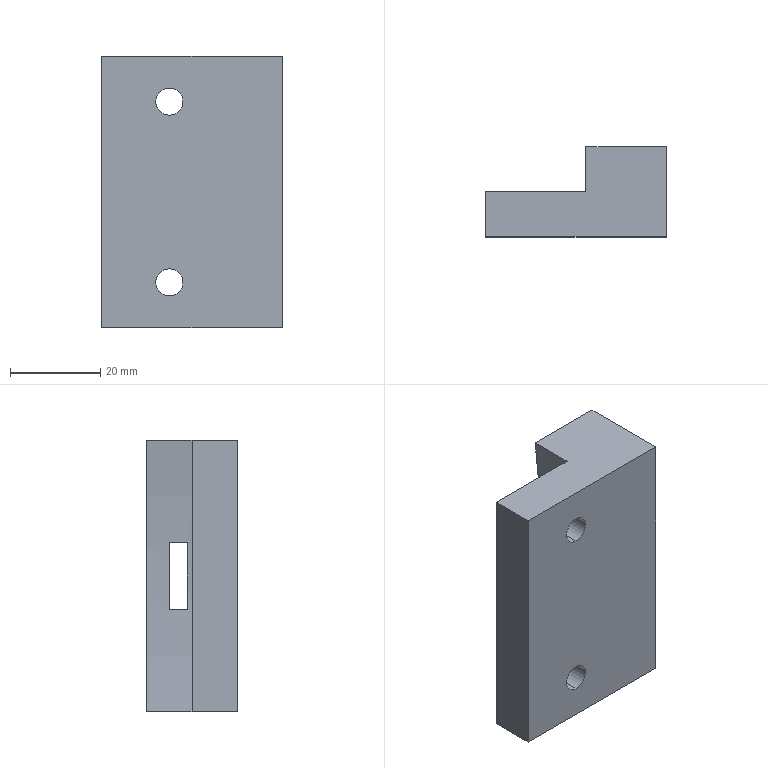Part | SolidWorks | features ICE 3, Extrusion 1 | 1 solid | 16 faces | box 40 x 20 x 60 mm | volume 32417 mm3 | plane 11 | cylinder 5 | commonest cylinder face diameters 6 x4 490 x1
STEP:
#1=CARTESIAN_POINT('',(15.,-20.,7.));
#2=VERTEX_POINT('',#1);
#3=CARTESIAN_POINT('',(15.,-20.,13.));
#4=VERTEX_POINT('',#3);
#5=CARTESIAN_POINT('',(15.,-20.,10.));
#6=DIRECTION('',(0.,1.,0.));
#7=DIRECTION('',(0.,0.,1.));
#8=AXIS2_PLACEMENT_3D('',#5,#6,#7);
#9=CIRCLE('',#8,3.);
#10=EDGE_CURVE('',#2,#4,#9,.T.);
#11=ORIENTED_EDGE('',*,*,#10,.F.);
#12=CARTESIAN_POINT('',(15.,-10.,7.));
#13=VERTEX_POINT('',#12);
#14=CARTESIAN_POINT('',(15.,-20.,7.));
#15=DIRECTION('',(0.,1.,0.));
#16=VECTOR('',#15,1000.);
#17=LINE('',#14,#16);
#18=EDGE_CURVE('',#2,#13,#17,.T.);
#19=ORIENTED_EDGE('',*,*,#18,.T.);
#20=CARTESIAN_POINT('',(15.,-10.,13.));
#21=VERTEX_POINT('',#20);
#22=CARTESIAN_POINT('',(15.,-10.,10.));
#23=DIRECTION('',(0.,1.,0.));
#24=DIRECTION('',(0.,0.,1.));
#25=AXIS2_PLACEMENT_3D('',#22,#23,#24);
#26=CIRCLE('',#25,3.);
#27=EDGE_CURVE('',#13,#21,#26,.T.);
#28=ORIENTED_EDGE('',*,*,#27,.T.);
#29=CARTESIAN_POINT('',(15.,-20.,13.));
#30=DIRECTION('',(0.,1.,0.));
#31=VECTOR('',#30,1000.);
#32=LINE('',#29,#31);
#33=EDGE_CURVE('',#4,#21,#32,.T.);
#34=ORIENTED_EDGE('',*,*,#33,.F.);
#35=EDGE_LOOP('',(#11,#19,#28,#34));
#36=FACE_OUTER_BOUND('',#35,.T.);
#37=CARTESIAN_POINT('',(15.,-20.,10.));
#38=DIRECTION('',(0.,1.,0.));
#39=DIRECTION('',(0.,0.,1.));
#40=AXIS2_PLACEMENT_3D('',#37,#38,#39);
#41=CYLINDRICAL_SURFACE('',#40,3.);
#42=ADVANCED_FACE('',(#36),#41,.F.);
#43=CARTESIAN_POINT('',(15.,-20.,47.));
#44=VERTEX_POINT('',#43);
#45=CARTESIAN_POINT('',(15.,-20.,53.));
#46=VERTEX_POINT('',#45);
#47=CARTESIAN_POINT('',(15.,-20.,50.));
#48=DIRECTION('',(0.,1.,0.));
#49=DIRECTION('',(0.,0.,1.));
#50=AXIS2_PLACEMENT_3D('',#47,#48,#49);
#51=CIRCLE('',#50,3.);
#52=EDGE_CURVE('',#44,#46,#51,.T.);
#53=ORIENTED_EDGE('',*,*,#52,.F.);
#54=CARTESIAN_POINT('',(15.,-10.,47.));
#55=VERTEX_POINT('',#54);
#56=CARTESIAN_POINT('',(15.,-20.,47.));
#57=DIRECTION('',(0.,1.,0.));
#58=VECTOR('',#57,1000.);
#59=LINE('',#56,#58);
#60=EDGE_CURVE('',#44,#55,#59,.T.);
#61=ORIENTED_EDGE('',*,*,#60,.T.);
#62=CARTESIAN_POINT('',(15.,-10.,53.));
#63=VERTEX_POINT('',#62);
#64=CARTESIAN_POINT('',(15.,-10.,50.));
#65=DIRECTION('',(0.,1.,0.));
#66=DIRECTION('',(0.,0.,1.));
#67=AXIS2_PLACEMENT_3D('',#64,#65,#66);
#68=CIRCLE('',#67,3.);
#69=EDGE_CURVE('',#55,#63,#68,.T.);
#70=ORIENTED_EDGE('',*,*,#69,.T.);
#71=CARTESIAN_POINT('',(15.,-20.,53.));
#72=DIRECTION('',(0.,1.,0.));
#73=VECTOR('',#72,1000.);
#74=LINE('',#71,#73);
#75=EDGE_CURVE('',#46,#63,#74,.T.);
#76=ORIENTED_EDGE('',*,*,#75,.F.);
#77=EDGE_LOOP('',(#53,#61,#70,#76));
#78=FACE_OUTER_BOUND('',#77,.T.);
#79=CARTESIAN_POINT('',(15.,-20.,50.));
#80=DIRECTION('',(0.,1.,0.));
#81=DIRECTION('',(0.,0.,1.));
#82=AXIS2_PLACEMENT_3D('',#79,#80,#81);
#83=CYLINDRICAL_SURFACE('',#82,3.);
#84=ADVANCED_FACE('',(#78),#83,.F.);
#85=CARTESIAN_POINT('',(40.,0.,0.));
#86=VERTEX_POINT('',#85);
#87=CARTESIAN_POINT('',(22.2,0.,0.));
#88=VERTEX_POINT('',#87);
#89=CARTESIAN_POINT('',(40.,0.,0.));
#90=DIRECTION('',(-1.,0.,0.));
#91=VECTOR('',#90,1000.);
#92=LINE('',#89,#91);
#93=EDGE_CURVE('',#86,#88,#92,.T.);
#94=ORIENTED_EDGE('',*,*,#93,.T.);
#95=CARTESIAN_POINT('',(22.2,0.,60.));
#96=VERTEX_POINT('',#95);
#97=CARTESIAN_POINT('',(-220.956,0.,30.));
#98=DIRECTION('',(0.,1.,0.));
#99=DIRECTION('',(0.,0.,-1.));
#100=AXIS2_PLACEMENT_3D('',#97,#98,#99);
#101=CIRCLE('',#100,245.);
#102=EDGE_CURVE('',#96,#88,#101,.T.);
#103=ORIENTED_EDGE('',*,*,#102,.F.);
#104=CARTESIAN_POINT('',(40.,0.,60.));
#105=VERTEX_POINT('',#104);
#106=CARTESIAN_POINT('',(40.,0.,60.));
#107=DIRECTION('',(-1.,0.,0.));
#108=VECTOR('',#107,1000.);
#109=LINE('',#106,#108);
#110=EDGE_CURVE('',#105,#96,#109,.T.);
#111=ORIENTED_EDGE('',*,*,#110,.F.);
#112=CARTESIAN_POINT('',(40.,0.,60.));
#113=DIRECTION('',(0.,0.,-1.));
#114=VECTOR('',#113,1000.);
#115=LINE('',#112,#114);
#116=EDGE_CURVE('',#105,#86,#115,.T.);
#117=ORIENTED_EDGE('',*,*,#116,.T.);
#118=EDGE_LOOP('',(#94,#103,#111,#117));
#119=FACE_OUTER_BOUND('',#118,.T.);
#120=CARTESIAN_POINT('',(40.,0.,60.));
#121=DIRECTION('',(0.,-1.,0.));
#122=DIRECTION('',(0.,0.,-1.));
#123=AXIS2_PLACEMENT_3D('',#120,#121,#122);
#124=PLANE('',#123);
#125=ADVANCED_FACE('',(#119),#124,.F.);
#126=CARTESIAN_POINT('',(0.,-10.,60.));
#127=VERTEX_POINT('',#126);
#128=CARTESIAN_POINT('',(0.,-20.,60.));
#129=VERTEX_POINT('',#128);
#130=CARTESIAN_POINT('',(0.,0.,60.));
#131=DIRECTION('',(0.,-1.,0.));
#132=VECTOR('',#131,1000.);
#133=LINE('',#130,#132);
#134=EDGE_CURVE('',#127,#129,#133,.T.);
#135=ORIENTED_EDGE('',*,*,#134,.F.);
#136=CARTESIAN_POINT('',(0.,-10.,0.));
#137=VERTEX_POINT('',#136);
#138=CARTESIAN_POINT('',(0.,-10.,0.));
#139=DIRECTION('',(0.,0.,1.));
#140=VECTOR('',#139,1000.);
#141=LINE('',#138,#140);
#142=EDGE_CURVE('',#137,#127,#141,.T.);
#143=ORIENTED_EDGE('',*,*,#142,.F.);
#144=CARTESIAN_POINT('',(0.,-20.,0.));
#145=VERTEX_POINT('',#144);
#146=CARTESIAN_POINT('',(0.,0.,0.));
#147=DIRECTION('',(0.,-1.,0.));
#148=VECTOR('',#147,1000.);
#149=LINE('',#146,#148);
#150=EDGE_CURVE('',#137,#145,#149,.T.);
#151=ORIENTED_EDGE('',*,*,#150,.T.);
#152=CARTESIAN_POINT('',(0.,-20.,60.));
#153=DIRECTION('',(0.,0.,-1.));
#154=VECTOR('',#153,1000.);
#155=LINE('',#152,#154);
#156=EDGE_CURVE('',#129,#145,#155,.T.);
#157=ORIENTED_EDGE('',*,*,#156,.F.);
#158=EDGE_LOOP('',(#135,#143,#151,#157));
#159=FACE_OUTER_BOUND('',#158,.T.);
#160=CARTESIAN_POINT('',(0.,0.,60.));
#161=DIRECTION('',(1.,0.,0.));
#162=DIRECTION('',(0.,0.,-1.));
#163=AXIS2_PLACEMENT_3D('',#160,#161,#162);
#164=PLANE('',#163);
#165=ADVANCED_FACE('',(#159),#164,.F.);
#166=CARTESIAN_POINT('',(15.,-20.,10.));
#167=DIRECTION('',(0.,1.,0.));
#168=DIRECTION('',(0.,0.,1.));
#169=AXIS2_PLACEMENT_3D('',#166,#167,#168);
#170=CIRCLE('',#169,3.);
#171=EDGE_CURVE('',#4,#2,#170,.T.);
#172=ORIENTED_EDGE('',*,*,#171,.T.);
#173=ORIENTED_EDGE('',*,*,#10,.T.);
#174=EDGE_LOOP('',(#172,#173));
#175=FACE_BOUND('',#174,.T.);
#176=CARTESIAN_POINT('',(15.,-20.,50.));
#177=DIRECTION('',(0.,1.,0.));
#178=DIRECTION('',(0.,0.,1.));
#179=AXIS2_PLACEMENT_3D('',#176,#177,#178);
#180=CIRCLE('',#179,3.);
#181=EDGE_CURVE('',#46,#44,#180,.T.);
#182=ORIENTED_EDGE('',*,*,#181,.T.);
#183=ORIENTED_EDGE('',*,*,#52,.T.);
#184=EDGE_LOOP('',(#182,#183));
#185=FACE_BOUND('',#184,.T.);
#186=CARTESIAN_POINT('',(40.,-20.,0.));
#187=VERTEX_POINT('',#186);
#188=CARTESIAN_POINT('',(0.,-20.,0.));
#189=DIRECTION('',(1.,0.,0.));
#190=VECTOR('',#189,1000.);
#191=LINE('',#188,#190);
#192=EDGE_CURVE('',#145,#187,#191,.T.);
#193=ORIENTED_EDGE('',*,*,#192,.T.);
#194=CARTESIAN_POINT('',(40.,-20.,60.));
#195=VERTEX_POINT('',#194);
#196=CARTESIAN_POINT('',(40.,-20.,60.));
#197=DIRECTION('',(0.,0.,-1.));
#198=VECTOR('',#197,1000.);
#199=LINE('',#196,#198);
#200=EDGE_CURVE('',#195,#187,#199,.T.);
#201=ORIENTED_EDGE('',*,*,#200,.F.);
#202=CARTESIAN_POINT('',(0.,-20.,60.));
#203=DIRECTION('',(1.,0.,0.));
#204=VECTOR('',#203,1000.);
#205=LINE('',#202,#204);
#206=EDGE_CURVE('',#129,#195,#205,.T.);
#207=ORIENTED_EDGE('',*,*,#206,.F.);
#208=ORIENTED_EDGE('',*,*,#156,.T.);
#209=EDGE_LOOP('',(#193,#201,#207,#208));
#210=FACE_OUTER_BOUND('',#209,.T.);
#211=CARTESIAN_POINT('',(0.,-20.,60.));
#212=DIRECTION('',(0.,1.,0.));
#213=DIRECTION('',(0.,0.,1.));
#214=AXIS2_PLACEMENT_3D('',#211,#212,#213);
#215=PLANE('',#214);
#216=ADVANCED_FACE('',(#175,#185,#210),#215,.F.);
#217=CARTESIAN_POINT('',(40.,-5.,22.5));
#218=VERTEX_POINT('',#217);
#219=CARTESIAN_POINT('',(40.,-5.,37.5));
#220=VERTEX_POINT('',#219);
#221=CARTESIAN_POINT('',(40.,-5.,37.5));
#222=DIRECTION('',(0.,0.,1.));
#223=VECTOR('',#222,1000.);
#224=LINE('',#221,#223);
#225=EDGE_CURVE('',#218,#220,#224,.T.);
#226=ORIENTED_EDGE('',*,*,#225,.F.);
#227=CARTESIAN_POINT('',(40.,-9.,22.5));
#228=VERTEX_POINT('',#227);
#229=CARTESIAN_POINT('',(40.,-5.,22.5));
#230=DIRECTION('',(0.,1.,0.));
#231=VECTOR('',#230,1000.);
#232=LINE('',#229,#231);
#233=EDGE_CURVE('',#228,#218,#232,.T.);
#234=ORIENTED_EDGE('',*,*,#233,.F.);
#235=CARTESIAN_POINT('',(40.,-9.,37.5));
#236=VERTEX_POINT('',#235);
#237=CARTESIAN_POINT('',(40.,-9.,37.5));
#238=DIRECTION('',(0.,0.,-1.));
#239=VECTOR('',#238,1000.);
#240=LINE('',#237,#239);
#241=EDGE_CURVE('',#236,#228,#240,.T.);
#242=ORIENTED_EDGE('',*,*,#241,.F.);
#243=CARTESIAN_POINT('',(40.,-5.,37.5));
#244=DIRECTION('',(0.,-1.,0.));
#245=VECTOR('',#244,1000.);
#246=LINE('',#243,#245);
#247=EDGE_CURVE('',#220,#236,#246,.T.);
#248=ORIENTED_EDGE('',*,*,#247,.F.);
#249=EDGE_LOOP('',(#226,#234,#242,#248));
#250=FACE_BOUND('',#249,.T.);
#251=CARTESIAN_POINT('',(40.,-20.,0.));
#252=DIRECTION('',(0.,1.,0.));
#253=VECTOR('',#252,1000.);
#254=LINE('',#251,#253);
#255=EDGE_CURVE('',#187,#86,#254,.T.);
#256=ORIENTED_EDGE('',*,*,#255,.T.);
#257=ORIENTED_EDGE('',*,*,#116,.F.);
#258=CARTESIAN_POINT('',(40.,-20.,60.));
#259=DIRECTION('',(0.,1.,0.));
#260=VECTOR('',#259,1000.);
#261=LINE('',#258,#260);
#262=EDGE_CURVE('',#195,#105,#261,.T.);
#263=ORIENTED_EDGE('',*,*,#262,.F.);
#264=ORIENTED_EDGE('',*,*,#200,.T.);
#265=EDGE_LOOP('',(#256,#257,#263,#264));
#266=FACE_OUTER_BOUND('',#265,.T.);
#267=CARTESIAN_POINT('',(40.,-20.,60.));
#268=DIRECTION('',(-1.,0.,0.));
#269=DIRECTION('',(0.,0.,1.));
#270=AXIS2_PLACEMENT_3D('',#267,#268,#269);
#271=PLANE('',#270);
#272=ADVANCED_FACE('',(#250,#266),#271,.F.);
#273=CARTESIAN_POINT('',(22.2,-10.,60.));
#274=VERTEX_POINT('',#273);
#275=CARTESIAN_POINT('',(22.2,-10.,60.));
#276=DIRECTION('',(0.,1.,0.));
#277=VECTOR('',#276,1000.);
#278=LINE('',#275,#277);
#279=EDGE_CURVE('',#274,#96,#278,.T.);
#280=ORIENTED_EDGE('',*,*,#279,.F.);
#281=CARTESIAN_POINT('',(0.,-10.,60.));
#282=DIRECTION('',(1.,0.,0.));
#283=VECTOR('',#282,1000.);
#284=LINE('',#281,#283);
#285=EDGE_CURVE('',#127,#274,#284,.T.);
#286=ORIENTED_EDGE('',*,*,#285,.F.);
#287=ORIENTED_EDGE('',*,*,#134,.T.);
#288=ORIENTED_EDGE('',*,*,#206,.T.);
#289=ORIENTED_EDGE('',*,*,#262,.T.);
#290=ORIENTED_EDGE('',*,*,#110,.T.);
#291=EDGE_LOOP('',(#280,#286,#287,#288,#289,#290));
#292=FACE_OUTER_BOUND('',#291,.T.);
#293=CARTESIAN_POINT('',(0.,0.,60.));
#294=DIRECTION('',(0.,0.,1.));
#295=DIRECTION('',(1.,0.,0.));
#296=AXIS2_PLACEMENT_3D('',#293,#294,#295);
#297=PLANE('',#296);
#298=ADVANCED_FACE('',(#292),#297,.T.);
#299=CARTESIAN_POINT('',(22.2,-10.,0.));
#300=VERTEX_POINT('',#299);
#301=CARTESIAN_POINT('',(22.2,-10.,0.));
#302=DIRECTION('',(-1.,0.,0.));
#303=VECTOR('',#302,1000.);
#304=LINE('',#301,#303);
#305=EDGE_CURVE('',#300,#137,#304,.T.);
#306=ORIENTED_EDGE('',*,*,#305,.F.);
#307=CARTESIAN_POINT('',(22.2,-10.,0.));
#308=DIRECTION('',(0.,1.,0.));
#309=VECTOR('',#308,1000.);
#310=LINE('',#307,#309);
#311=EDGE_CURVE('',#300,#88,#310,.T.);
#312=ORIENTED_EDGE('',*,*,#311,.T.);
#313=ORIENTED_EDGE('',*,*,#93,.F.);
#314=ORIENTED_EDGE('',*,*,#255,.F.);
#315=ORIENTED_EDGE('',*,*,#192,.F.);
#316=ORIENTED_EDGE('',*,*,#150,.F.);
#317=EDGE_LOOP('',(#306,#312,#313,#314,#315,#316));
#318=FACE_OUTER_BOUND('',#317,.T.);
#319=CARTESIAN_POINT('',(0.,0.,0.));
#320=DIRECTION('',(0.,0.,1.));
#321=DIRECTION('',(1.,0.,0.));
#322=AXIS2_PLACEMENT_3D('',#319,#320,#321);
#323=PLANE('',#322);
#324=ADVANCED_FACE('',(#318),#323,.F.);
#325=CARTESIAN_POINT('',(23.929,-9.,37.5));
#326=VERTEX_POINT('',#325);
#327=CARTESIAN_POINT('',(23.929,-9.,22.5));
#328=VERTEX_POINT('',#327);
#329=CARTESIAN_POINT('',(-220.956,-9.,30.));
#330=DIRECTION('',(0.,1.,0.));
#331=DIRECTION('',(0.,0.,-1.));
#332=AXIS2_PLACEMENT_3D('',#329,#330,#331);
#333=CIRCLE('',#332,245.);
#334=EDGE_CURVE('',#326,#328,#333,.T.);
#335=ORIENTED_EDGE('',*,*,#334,.T.);
#336=CARTESIAN_POINT('',(23.929,-5.,22.5));
#337=VERTEX_POINT('',#336);
#338=CARTESIAN_POINT('',(23.929,-10.,22.5));
#339=DIRECTION('',(0.,1.,0.));
#340=VECTOR('',#339,1000.);
#341=LINE('',#338,#340);
#342=EDGE_CURVE('',#328,#337,#341,.T.);
#343=ORIENTED_EDGE('',*,*,#342,.T.);
#344=CARTESIAN_POINT('',(23.929,-5.,37.5));
#345=VERTEX_POINT('',#344);
#346=CARTESIAN_POINT('',(-220.956,-5.,30.));
#347=DIRECTION('',(0.,-1.,0.));
#348=DIRECTION('',(0.,0.,1.));
#349=AXIS2_PLACEMENT_3D('',#346,#347,#348);
#350=CIRCLE('',#349,245.);
#351=EDGE_CURVE('',#337,#345,#350,.T.);
#352=ORIENTED_EDGE('',*,*,#351,.T.);
#353=CARTESIAN_POINT('',(23.929,-10.,37.5));
#354=DIRECTION('',(0.,-1.,0.));
#355=VECTOR('',#354,1000.);
#356=LINE('',#353,#355);
#357=EDGE_CURVE('',#345,#326,#356,.T.);
#358=ORIENTED_EDGE('',*,*,#357,.T.);
#359=EDGE_LOOP('',(#335,#343,#352,#358));
#360=FACE_BOUND('',#359,.T.);
#361=ORIENTED_EDGE('',*,*,#102,.T.);
#362=ORIENTED_EDGE('',*,*,#311,.F.);
#363=CARTESIAN_POINT('',(-220.956,-10.,30.));
#364=DIRECTION('',(0.,1.,0.));
#365=DIRECTION('',(0.,0.,-1.));
#366=AXIS2_PLACEMENT_3D('',#363,#364,#365);
#367=CIRCLE('',#366,245.);
#368=EDGE_CURVE('',#274,#300,#367,.T.);
#369=ORIENTED_EDGE('',*,*,#368,.F.);
#370=ORIENTED_EDGE('',*,*,#279,.T.);
#371=EDGE_LOOP('',(#361,#362,#369,#370));
#372=FACE_OUTER_BOUND('',#371,.T.);
#373=CARTESIAN_POINT('',(-220.956,-10.,30.));
#374=DIRECTION('',(0.,1.,0.));
#375=DIRECTION('',(0.,0.,1.));
#376=AXIS2_PLACEMENT_3D('',#373,#374,#375);
#377=CYLINDRICAL_SURFACE('',#376,245.);
#378=ADVANCED_FACE('',(#360,#372),#377,.F.);
#379=CARTESIAN_POINT('',(15.,-10.,10.));
#380=DIRECTION('',(0.,1.,0.));
#381=DIRECTION('',(0.,0.,1.));
#382=AXIS2_PLACEMENT_3D('',#379,#380,#381);
#383=CIRCLE('',#382,3.);
#384=EDGE_CURVE('',#21,#13,#383,.T.);
#385=ORIENTED_EDGE('',*,*,#384,.F.);
#386=ORIENTED_EDGE('',*,*,#27,.F.);
#387=EDGE_LOOP('',(#385,#386));
#388=FACE_BOUND('',#387,.T.);
#389=CARTESIAN_POINT('',(15.,-10.,50.));
#390=DIRECTION('',(0.,1.,0.));
#391=DIRECTION('',(0.,0.,1.));
#392=AXIS2_PLACEMENT_3D('',#389,#390,#391);
#393=CIRCLE('',#392,3.);
#394=EDGE_CURVE('',#63,#55,#393,.T.);
#395=ORIENTED_EDGE('',*,*,#394,.F.);
#396=ORIENTED_EDGE('',*,*,#69,.F.);
#397=EDGE_LOOP('',(#395,#396));
#398=FACE_BOUND('',#397,.T.);
#399=ORIENTED_EDGE('',*,*,#368,.T.);
#400=ORIENTED_EDGE('',*,*,#305,.T.);
#401=ORIENTED_EDGE('',*,*,#142,.T.);
#402=ORIENTED_EDGE('',*,*,#285,.T.);
#403=EDGE_LOOP('',(#399,#400,#401,#402));
#404=FACE_OUTER_BOUND('',#403,.T.);
#405=CARTESIAN_POINT('',(-220.956,-10.,30.));
#406=DIRECTION('',(0.,-1.,0.));
#407=DIRECTION('',(0.,0.,-1.));
#408=AXIS2_PLACEMENT_3D('',#405,#406,#407);
#409=PLANE('',#408);
#410=ADVANCED_FACE('',(#388,#398,#404),#409,.F.);
#411=ORIENTED_EDGE('',*,*,#60,.F.);
#412=ORIENTED_EDGE('',*,*,#181,.F.);
#413=ORIENTED_EDGE('',*,*,#75,.T.);
#414=ORIENTED_EDGE('',*,*,#394,.T.);
#415=EDGE_LOOP('',(#411,#412,#413,#414));
#416=FACE_OUTER_BOUND('',#415,.T.);
#417=CARTESIAN_POINT('',(15.,-20.,50.));
#418=DIRECTION('',(0.,1.,0.));
#419=DIRECTION('',(0.,0.,1.));
#420=AXIS2_PLACEMENT_3D('',#417,#418,#419);
#421=CYLINDRICAL_SURFACE('',#420,3.);
#422=ADVANCED_FACE('',(#416),#421,.F.);
#423=ORIENTED_EDGE('',*,*,#18,.F.);
#424=ORIENTED_EDGE('',*,*,#171,.F.);
#425=ORIENTED_EDGE('',*,*,#33,.T.);
#426=ORIENTED_EDGE('',*,*,#384,.T.);
#427=EDGE_LOOP('',(#423,#424,#425,#426));
#428=FACE_OUTER_BOUND('',#427,.T.);
#429=CARTESIAN_POINT('',(15.,-20.,10.));
#430=DIRECTION('',(0.,1.,0.));
#431=DIRECTION('',(0.,0.,1.));
#432=AXIS2_PLACEMENT_3D('',#429,#430,#431);
#433=CYLINDRICAL_SURFACE('',#432,3.);
#434=ADVANCED_FACE('',(#428),#433,.F.);
#435=CARTESIAN_POINT('',(-9.,-9.,22.5));
#436=DIRECTION('',(1.,0.,0.));
#437=VECTOR('',#436,1000.);
#438=LINE('',#435,#437);
#439=EDGE_CURVE('',#328,#228,#438,.T.);
#440=ORIENTED_EDGE('',*,*,#439,.T.);
#441=ORIENTED_EDGE('',*,*,#233,.T.);
#442=CARTESIAN_POINT('',(-9.,-5.,22.5));
#443=DIRECTION('',(1.,0.,0.));
#444=VECTOR('',#443,1000.);
#445=LINE('',#442,#444);
#446=EDGE_CURVE('',#337,#218,#445,.T.);
#447=ORIENTED_EDGE('',*,*,#446,.F.);
#448=ORIENTED_EDGE('',*,*,#342,.F.);
#449=EDGE_LOOP('',(#440,#441,#447,#448));
#450=FACE_OUTER_BOUND('',#449,.T.);
#451=CARTESIAN_POINT('',(-9.,-5.,22.5));
#452=DIRECTION('',(0.,0.,-1.));
#453=DIRECTION('',(-1.,0.,0.));
#454=AXIS2_PLACEMENT_3D('',#451,#452,#453);
#455=PLANE('',#454);
#456=ADVANCED_FACE('',(#450),#455,.F.);
#457=CARTESIAN_POINT('',(-9.,-9.,37.5));
#458=DIRECTION('',(1.,0.,0.));
#459=VECTOR('',#458,1000.);
#460=LINE('',#457,#459);
#461=EDGE_CURVE('',#326,#236,#460,.T.);
#462=ORIENTED_EDGE('',*,*,#461,.T.);
#463=ORIENTED_EDGE('',*,*,#241,.T.);
#464=ORIENTED_EDGE('',*,*,#439,.F.);
#465=ORIENTED_EDGE('',*,*,#334,.F.);
#466=EDGE_LOOP('',(#462,#463,#464,#465));
#467=FACE_OUTER_BOUND('',#466,.T.);
#468=CARTESIAN_POINT('',(-9.,-9.,37.5));
#469=DIRECTION('',(0.,-1.,0.));
#470=DIRECTION('',(0.,0.,-1.));
#471=AXIS2_PLACEMENT_3D('',#468,#469,#470);
#472=PLANE('',#471);
#473=ADVANCED_FACE('',(#467),#472,.F.);
#474=CARTESIAN_POINT('',(-9.,-5.,37.5));
#475=DIRECTION('',(1.,0.,0.));
#476=VECTOR('',#475,1000.);
#477=LINE('',#474,#476);
#478=EDGE_CURVE('',#345,#220,#477,.T.);
#479=ORIENTED_EDGE('',*,*,#478,.T.);
#480=ORIENTED_EDGE('',*,*,#247,.T.);
#481=ORIENTED_EDGE('',*,*,#461,.F.);
#482=ORIENTED_EDGE('',*,*,#357,.F.);
#483=EDGE_LOOP('',(#479,#480,#481,#482));
#484=FACE_OUTER_BOUND('',#483,.T.);
#485=CARTESIAN_POINT('',(-9.,-5.,37.5));
#486=DIRECTION('',(0.,0.,1.));
#487=DIRECTION('',(1.,0.,0.));
#488=AXIS2_PLACEMENT_3D('',#485,#486,#487);
#489=PLANE('',#488);
#490=ADVANCED_FACE('',(#484),#489,.F.);
#491=ORIENTED_EDGE('',*,*,#446,.T.);
#492=ORIENTED_EDGE('',*,*,#225,.T.);
#493=ORIENTED_EDGE('',*,*,#478,.F.);
#494=ORIENTED_EDGE('',*,*,#351,.F.);
#495=EDGE_LOOP('',(#491,#492,#493,#494));
#496=FACE_OUTER_BOUND('',#495,.T.);
#497=CARTESIAN_POINT('',(-9.,-5.,37.5));
#498=DIRECTION('',(0.,1.,0.));
#499=DIRECTION('',(0.,0.,1.));
#500=AXIS2_PLACEMENT_3D('',#497,#498,#499);
#501=PLANE('',#500);
#502=ADVANCED_FACE('',(#496),#501,.F.);
#503=CLOSED_SHELL('',(#42,#84,#125,#165,#216,#272,#298,#324,#378,#410,#422,#434,#456,#473,#490,#502));
#504=MANIFOLD_SOLID_BREP('',#503);
#505=CARTESIAN_POINT('',(0.,0.,0.));
#506=DIRECTION('',(0.,0.,1.));
#507=DIRECTION('',(1.,0.,0.));
#508=AXIS2_PLACEMENT_3D('',#505,#506,#507);
#509=(LENGTH_UNIT()NAMED_UNIT(*)SI_UNIT(.MILLI.,.METRE.));
#510=UNCERTAINTY_MEASURE_WITH_UNIT(LENGTH_MEASURE(0.00001),#509,'','');
#511=(NAMED_UNIT(*)PLANE_ANGLE_UNIT()SI_UNIT($,.RADIAN.));
#512=(NAMED_UNIT(*)SI_UNIT($,.STERADIAN.)SOLID_ANGLE_UNIT());
#513=(GEOMETRIC_REPRESENTATION_CONTEXT(3)GLOBAL_UNCERTAINTY_ASSIGNED_CONTEXT((#510))GLOBAL_UNIT_ASSIGNED_CONTEXT((#509,#511,#512))REPRESENTATION_CONTEXT('',''));
#514=ADVANCED_BREP_SHAPE_REPRESENTATION('',(#504,#508),#513);